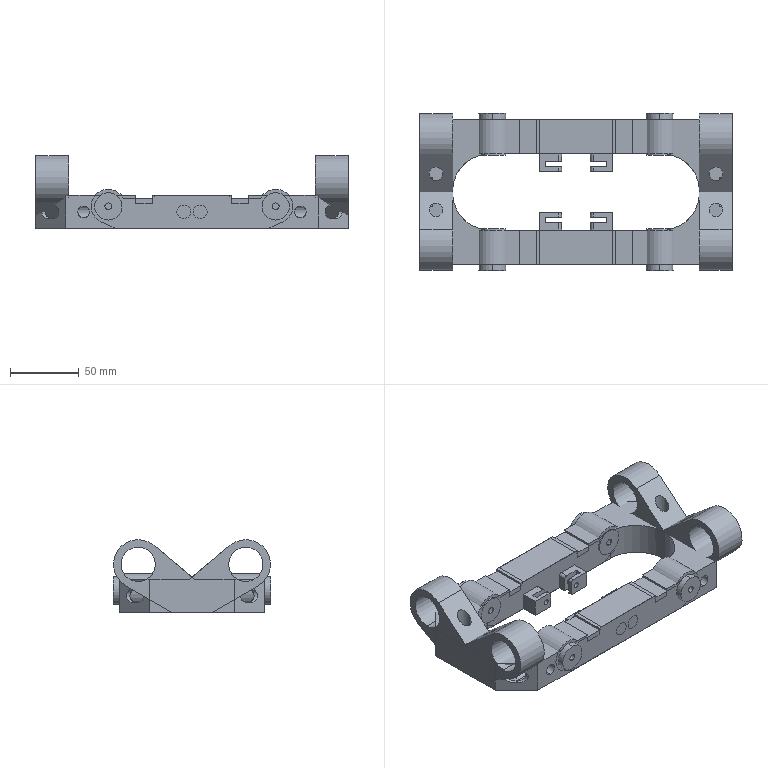CAM job | Mastercam | 3-axis milling, 5-axis milling, drilling, other | part box 228 x 114.503 x 53 mm | stock box 238 x 120 x 53 mm
Tools:
tool_number,name,type,diameter_mm,corner_radius_mm,flutes,flute_length_mm,overall_length_mm,shoulder_length_mm,holder_diameter_mm,length_offset,diameter_offset,default_rpm,default_feed_mm_min,default_plunge_mm_min,coolant
1,50 Slot Mill or Saw,slot mill,50,0,4,4,50,6,50,1,1,1000,150,600,COOL_OFF
1,2.5 Drill,drill,2.5,0,2,25,50,40,50,1,1,1200,70,600,COOL_OFF
2,4.2 Drill,drill,4.2,0,2,25,50,40,50,2,2,1000,100,600,COOL_OFF
2,4.1 Drill,drill,4.1,0,2,25,50,40,50,2,2,1500,100,600,COOL_OFF
3,10 Ball Mill / Bull Nose Mill,ball end mill,10,5,4,25,200,30,50,3,3,5000,1000,600,COOL_OFF
3,50 Flat End Mill,end mill,50,0,4,25,75,25,50,3,3,1400,200,600,COOL_OFF
4,4 Ball Mill / Bull Nose Mill,ball end mill,4,2,4,25,100,30,50,4,4,5000,1500,600,COOL_OFF
5,5 Drill,drill,5,0,2,25,50,40,50,5,5,1300,100,600,COOL_OFF
5,5 Drill,drill,5,0,2,25,50,40,50,5,5,1300,100,600,COOL_OFF
6,6 Flat End Mill,end mill,6,0,4,25,75,25,50,6,6,8000,3000,600,COOL_OFF
6,6 Flat End Mill,end mill,6,0,4,25,75,25,50,6,6,8000,3000,600,COOL_OFF
7,6 Chamfer Mill,chamfer mill,6,0,4,25,75,30,50,7,7,5000,1500,600,COOL_OFF
7,6 Chamfer Mill,chamfer mill,6,0,4,25,75,30,50,7,7,5000,1500,600,COOL_OFF
9,10 Drill,drill,10,0,2,25,200,40,50,9,9,1100,100,600,COOL_OFF
9,10 Drill,drill,10,0,2,25,200,40,50,9,9,1100,100,600,COOL_OFF
10,10 Flat End Mill,end mill,10,0,4,25,75,25,50,10,10,8500,6000,600,COOL_OFF
10,10 Flat End Mill,end mill,10,0,4,25,75,25,50,10,10,8500,6000,600,COOL_OFF
11,10 Drill,drill,10,0,2,25,200,40,50,11,11,600,80,600,COOL_OFF
11,10 Drill,drill,10,0,2,25,200,40,50,11,11,600,80,600,COOL_OFF
12,12 Flat End Mill,end mill,12,0,4,25,75,25,50,12,12,8000,6000,600,COOL_OFF
12,12 Flat End Mill,end mill,12,0,4,25,75,25,50,12,12,8000,6000,600,COOL_OFF
13,10 Bull Nose Mill,bull end mill,10,1,4,25,100,25,50,13,13,8000,4000,600,COOL_OFF
16,16 Flat End Mill,end mill,16,0,4,25,75,25,50,16,16,8250,4000,600,COOL_OFF
16,16 Flat End Mill,end mill,16,0,4,25,75,25,50,16,16,8250,4000,600,COOL_OFF
17,5 Ball Mill / Bull Nose Mill,ball end mill,5,2.5,4,25,100,30,50,17,17,5000,1500,600,COOL_OFF
17,5 Ball Mill / Bull Nose Mill,ball end mill,5,2.5,4,25,100,30,50,17,17,5000,1500,600,COOL_OFF
23,50 Flat End Mill,end mill,50,0,4,25,75,25,50,23,23,5000,4000,600,COOL_OFF
23,50 Flat End Mill,end mill,50,0,4,25,75,25,50,23,23,5000,4000,600,COOL_OFF
24,100 Flat End Mill,end mill,100,0,4,25,75,25,50,24,24,4000,1200,600,COOL_OFF
24,100 Flat End Mill,end mill,100,0,4,25,75,25,50,24,24,4000,1200,600,COOL_OFF
Operations:
seq,operation,operation_type,tool_number,tool_name,tool_diameter_mm,spindle_rpm,feed_mm_min,plunge_mm_min,retract_mm_min,cycle_time_s,wcs,posted,nc_file
1,Facing - [WCS: Plane] - [Tplane: Plane],Facing,24,100 Flat End Mill,100,4000,1200,600,1200,38.489,Plane,yes,1.nc
2,2D High Speed (2D Dynamic Mill) - [WCS: Plane] - [Tplane: Plane],HighSpeed2D,16,16 Flat End Mill,16,8250,4000,600,1200,119.906,Plane,yes,1.nc
3,Contour (2D) - [WCS: Plane] - [Tplane: Plane],Contour,16,16 Flat End Mill,16,5000,1000,600,1200,92.313,Plane,yes,1.nc
4,Contour (2D chamfer) - [WCS: Plane] - [Tplane: Plane],Contour,7,6 Chamfer Mill,6,5000,1500,600,1200,28.973,Plane,yes,1.nc
5,Facing - [WCS: Plane-4] - [Tplane: Plane-4],Facing,24,100 Flat End Mill,100,5000,3000,600,1200,65.426,Plane-4,yes,1.nc
6,Facing - [WCS: Plane-4] - [Tplane: Plane-4],Facing,24,100 Flat End Mill,100,5000,1000,600,1200,46.149,Plane-4,yes,1.nc
7,Drill/Counterbore - [WCS: Plane-4] - [Tplane: Plane-4],Drill,7,6 Chamfer Mill,6,5000,300,600,1200,1.67,Plane-4,yes,1.nc
8,Peck Drill - [WCS: Plane-4] - [Tplane: Plane-4],Drill,11,10 Drill,10,1200,150,600,1200,47.946,Plane-4,yes,1.nc
9,Contour (2D chamfer) - [WCS: Plane-4] - [Tplane: Plane-4],Contour,7,6 Chamfer Mill,6,5000,1500,600,1200,33.878,Plane-4,yes,1.nc
10,Contour (2D) - [WCS: Plane-2] - [Tplane: Plane-2],Contour,23,50 Flat End Mill,50,5000,4000,600,1200,376.188,Plane-2,yes,1.nc
11,Contour (Remachining) - [WCS: Plane-2] - [Tplane: Plane-2],Contour,10,10 Flat End Mill,10,8000,4000,600,1200,22.001,Plane-2,yes,1.nc
12,Contour (2D) - [WCS: Plane-2] - [Tplane: Plane-2],Contour,10,10 Flat End Mill,10,6000,1000,600,1200,46.662,Plane-2,yes,1.nc
13,Contour (Ramp) - [WCS: Plane-2] - [Tplane: Plane-2],Contour,10,10 Flat End Mill,10,8000,4000,600,1200,56.103,Plane-2,yes,1.nc
14,Contour (Ramp) - [WCS: Plane-2] - [Tplane: Plane-2],Contour,10,10 Flat End Mill,10,8000,1000,600,1200,19.219,Plane-2,yes,1.nc
15,Drill/Counterbore - [WCS: Plane-2] - [Tplane: Plane-2],Drill,7,6 Chamfer Mill,6,5000,300,600,1200,0.835,Plane-2,yes,1.nc
16,Peck Drill - [WCS: Plane-2] - [Tplane: Plane-2],Drill,11,10 Drill,10,1000,100,600,1200,28.243,Plane-2,yes,1.nc
17,Manual Entry (G0G90G54X-300.),ManualEntry,,,,0,0,0,0,0,Plane,yes,1.nc
18,Peck Drill - [WCS: Plane-2] - [Tplane: Plane-2],Drill,9,10 Drill,10,600,80,600,1200,116.677,Plane-2,yes,1.nc
19,Manual Entry (G0G90G54X-300.),ManualEntry,,,,0,0,0,0,0,Plane,yes,1.nc
20,Contour (2D chamfer) - [WCS: Plane-2] - [Tplane: Plane-2],Contour,7,6 Chamfer Mill,6,5000,1500,600,1200,19.89,Plane-2,yes,1.nc
21,Transform/Rotate Rotate About Point/Toolplane/Geometry,XForm,,,,0,0,0,0,685.819,Plane-2,yes,1.nc
22,Stock model - [WCS: Top] - [Tplane: Plane] - 1,139,,,,0,0,0,0,0,Top,yes,1.nc|2.nc|3.nc
23,2D High Speed (2D Area Mill) - [WCS: Plane-3] - [Tplane: Plane-3],HighSpeed2D,12,12 Flat End Mill,12,8500,6000,600,1200,76.463,Plane-3,yes,1.nc
24,Contour (Ramp) - [WCS: Plane-3] - [Tplane: Plane-3],Contour,12,12 Flat End Mill,12,8000,6000,600,1200,6.551,Plane-3,yes,1.nc
25,Contour (2D) - [WCS: Plane-3] - [Tplane: Plane-3],Contour,12,12 Flat End Mill,12,8000,1000,600,1200,8.109,Plane-3,yes,1.nc
26,2D High Speed (2D Area Mill) - [WCS: Plane-3] - [Tplane: Plane-3],HighSpeed2D,12,12 Flat End Mill,12,8500,1500,600,1200,47.681,Plane-3,yes,1.nc
27,Drill/Counterbore - [WCS: Plane-3] - [Tplane: Plane-3],Drill,7,6 Chamfer Mill,6,5000,300,600,1200,3.381,Plane-3,yes,1.nc
28,Peck Drill - [WCS: Plane-3] - [Tplane: Plane-3],Drill,5,5 Drill,5,1300,100,600,1200,26.184,Plane-3,yes,1.nc
29,Peck Drill - [WCS: Plane-3] - [Tplane: Plane-3],Drill,11,10 Drill,10,600,80,600,1200,67.7,Plane-3,yes,1.nc
30,Peck Drill - [WCS: Plane-3] - [Tplane: Plane-3],Drill,11,10 Drill,10,1100,100,600,1200,14.333,Plane-3,yes,1.nc
31,Contour (Ramp) - [WCS: Plane-3] - [Tplane: Plane-3],Contour,6,6 Flat End Mill,6,8000,3000,600,1200,5.394,Plane-3,yes,1.nc
32,Contour (2D chamfer) - [WCS: Plane-3] - [Tplane: Plane-3],Contour,7,6 Chamfer Mill,6,5000,1500,600,1200,14.165,Plane-3,yes,1.nc
33,Contour (2D chamfer) - [WCS: Plane-3] - [Tplane: Plane-3],Contour,7,6 Chamfer Mill,6,5000,1500,600,1200,20.962,Plane-3,yes,1.nc
34,Transform/Rotate Rotate About Point/Toolplane/NCI,XForm,,,,0,0,0,0,290.923,Plane,yes,1.nc
35,Stock model - [WCS: Top] - [Tplane: Plane-3] - 2,139,,,,0,0,0,0,0,Top,yes,1.nc|2.nc|3.nc
36,Contour (Ramp) - [WCS: Plane-1] - [Tplane: Plane-1],Contour,23,50 Flat End Mill,50,5000,4000,600,1200,172.897,Plane-1,yes,1.nc
37,Contour (2D) - [WCS: Plane-1] - [Tplane: Plane-1],Contour,10,10 Flat End Mill,10,6000,1000,600,1200,25.422,Plane-1,yes,1.nc
38,Contour (Ramp) - [WCS: Plane-1] - [Tplane: Plane-1],Contour,6,6 Flat End Mill,6,8000,3000,600,1200,11.291,Plane-1,yes,1.nc
39,Contour (2D) - [WCS: Plane-1] - [Tplane: Plane-1],Contour,6,6 Flat End Mill,6,8000,1000,600,1200,12.906,Plane-1,yes,1.nc
40,Contour (2D chamfer) - [WCS: Plane-1] - [Tplane: Plane-1],Contour,7,6 Chamfer Mill,6,5000,1500,600,1200,13.542,Plane-1,yes,1.nc
41,Drill/Counterbore - [WCS: Plane-1] - [Tplane: Plane-1],Drill,7,6 Chamfer Mill,6,5000,300,600,1200,3.095,Plane-1,yes,1.nc
42,Stock model - [WCS: Top] - [Tplane: Plane-1] - 3,139,,,,0,0,0,0,0,Top,yes,1.nc|2.nc|3.nc
43,Contour (Ramp) - [WCS: Plane] - [Tplane: Plane],Contour,24,100 Flat End Mill,100,5000,4000,600,1200,242.961,Plane,yes,1.nc
44,2D High Speed (2D Area Mill) - [WCS: Plane] - [Tplane: Plane],HighSpeed2D,12,12 Flat End Mill,12,8500,5000,600,1200,251.096,Plane,yes,1.nc
45,2D High Speed (2D Area Mill) - [WCS: Plane] - [Tplane: Plane],HighSpeed2D,12,12 Flat End Mill,12,8500,1200,600,1200,126.788,Plane,yes,1.nc
46,Contour (Ramp) - [WCS: Plane] - [Tplane: Plane],Contour,10,10 Flat End Mill,10,8500,6000,600,1200,15.497,Plane,yes,1.nc
47,Contour (2D) - [WCS: Plane] - [Tplane: Plane],Contour,10,10 Flat End Mill,10,8500,1000,600,1200,11.429,Plane,yes,1.nc
48,Contour (Ramp) - [WCS: Plane] - [Tplane: Plane],Contour,12,12 Flat End Mill,12,8000,6000,600,1200,6.911,Plane,yes,1.nc
49,Contour (2D) - [WCS: Plane] - [Tplane: Plane],Contour,12,12 Flat End Mill,12,8000,1000,600,1200,11.582,Plane,yes,1.nc
50,Contour (2D chamfer) - [WCS: Plane] - [Tplane: Plane],Contour,7,6 Chamfer Mill,6,5000,1500,600,1200,8.268,Plane,yes,1.nc
51,Contour (2D chamfer) - [WCS: Plane] - [Tplane: Plane],Contour,7,6 Chamfer Mill,6,5000,1500,600,1200,12.882,Plane,yes,1.nc
52,Ruled - [WCS: Plane] - [Tplane: Plane],Ruled,12,12 Flat End Mill,12,8000,4000,2000,1200,23.404,Plane,yes,1.nc
53,Ruled - [WCS: Plane] - [Tplane: Plane],Ruled,12,12 Flat End Mill,12,8000,4000,2000,1200,23.404,Plane,yes,1.nc
54,Surface Finish Flowline - [WCS: Plane] - [Tplane: Plane],MultiSurfaceFinishFlowline,13,10 Bull Nose Mill,10,8000,4000,600,1200,77.618,Plane,yes,1.nc
55,Surface Finish Flowline - [WCS: Plane] - [Tplane: Plane],MultiSurfaceFinishFlowline,13,10 Bull Nose Mill,10,8000,4000,600,1200,77.618,Plane,yes,1.nc
56,Deburr 5-axis - [WCS: Plane] - [Tplane: Plane],459,17,5 Ball Mill / Bull Nose Mill,5,5000,1500,600,1200,29.492,Plane,yes,1.nc
57,Drill/Counterbore - [WCS: Plane] - [Tplane: Plane],Drill,7,6 Chamfer Mill,6,5000,300,600,1200,5.169,Plane,yes,1.nc
58,Stock model - [WCS: Top] - [Tplane: Plane] - 4,139,,,,0,0,0,0,0,Top,yes,1.nc|2.nc|3.nc
59,Contour (2D) - [WCS: Plane-5] - [Tplane: Plane-5],Contour,16,16 Flat End Mill,16,5000,1000,600,1200,49.081,Plane-5,yes,1.nc
60,Contour (2D) - [WCS: Plane-5] - [Tplane: Plane-4],Contour,16,16 Flat End Mill,16,6000,4000,600,1200,326.038,Plane-5,yes,1.nc
61,Contour (2D) - [WCS: Plane-5] - [Tplane: Plane-4],Contour,16,16 Flat End Mill,16,6000,1000,600,1200,63.018,Plane-5,yes,1.nc
62,Contour (Ramp) - [WCS: Plane-5] - [Tplane: Plane-4],Contour,16,16 Flat End Mill,16,6000,4000,600,1200,259.668,Plane-5,yes,1.nc
63,Deburr 5-axis - [WCS: Plane-5] - [Tplane: Plane-5],459,17,5 Ball Mill / Bull Nose Mill,5,5000,1500,600,1200,22.138,Plane-5,yes,1.nc
64,Stock model - [WCS: Top] - [Tplane: Plane-4] - 5,139,,,,0,0,0,0,0,Top,yes,1.nc|2.nc|3.nc
65,Facing - [WCS: Plane-4] - [Tplane: Plane-4],Facing,24,100 Flat End Mill,100,5000,3000,600,1200,65.426,Plane-4,yes,1.nc
66,Facing - [WCS: Plane-4] - [Tplane: Plane-4],Facing,24,100 Flat End Mill,100,5000,1000,600,1200,46.149,Plane-4,yes,1.nc
67,Drill/Counterbore - [WCS: Plane-4] - [Tplane: Plane-4],Drill,7,6 Chamfer Mill,6,5000,300,600,1200,1.67,Plane-4,yes,1.nc
68,Peck Drill - [WCS: Plane-4] - [Tplane: Plane-4],Drill,11,10 Drill,10,1200,150,600,1200,47.946,Plane-4,yes,1.nc
69,Contour (2D chamfer) - [WCS: Plane-4] - [Tplane: Plane-4],Contour,7,6 Chamfer Mill,6,5000,1500,600,1200,33.878,Plane-4,yes,1.nc
70,Contour (Ramp) - [WCS: Plane-2] - [Tplane: Plane-2],Contour,23,50 Flat End Mill,50,5000,4000,600,1200,356.8,Plane-2,yes,1.nc
71,Contour (Remachining) - [WCS: Plane-2] - [Tplane: Plane-2],Contour,10,10 Flat End Mill,10,8000,4000,600,1200,21.855,Plane-2,yes,1.nc
72,Contour (2D) - [WCS: Plane-2] - [Tplane: Plane-2],Contour,10,10 Flat End Mill,10,6000,1000,600,1200,46.67,Plane-2,yes,1.nc
73,Contour (Ramp) - [WCS: Plane-2] - [Tplane: Plane-2],Contour,10,10 Flat End Mill,10,8000,4000,600,1200,56.103,Plane-2,yes,1.nc
74,Contour (Ramp) - [WCS: Plane-2] - [Tplane: Plane-2],Contour,10,10 Flat End Mill,10,8000,1000,600,1200,19.219,Plane-2,yes,1.nc
75,Drill/Counterbore - [WCS: Plane-2] - [Tplane: Plane-2],Drill,7,6 Chamfer Mill,6,5000,300,600,1200,0.835,Plane-2,yes,1.nc
76,Peck Drill - [WCS: Plane-2] - [Tplane: Plane-2],Drill,11,10 Drill,10,1000,100,600,1200,28.243,Plane-2,yes,1.nc
77,Manual Entry (G0G90G54X-300.),ManualEntry,,,,0,0,0,0,0,Plane,yes,1.nc
78,Peck Drill - [WCS: Plane-2] - [Tplane: Plane-2],Drill,9,10 Drill,10,600,80,600,1200,116.677,Plane-2,yes,1.nc
79,Manual Entry (G0G90G54X-300.),ManualEntry,,,,0,0,0,0,0,Plane,yes,1.nc
80,Contour (2D chamfer) - [WCS: Plane-2] - [Tplane: Plane-2],Contour,7,6 Chamfer Mill,6,5000,1500,600,1200,19.89,Plane-2,yes,1.nc
81,2D High Speed (2D Area Mill) - [WCS: Plane-3] - [Tplane: Plane-3],HighSpeed2D,12,12 Flat End Mill,12,8500,6000,600,1200,76.465,Plane-3,yes,1.nc
82,Contour (Ramp) - [WCS: Plane-3] - [Tplane: Plane-3],Contour,12,12 Flat End Mill,12,8000,6000,600,1200,6.551,Plane-3,yes,1.nc
83,Contour (2D) - [WCS: Plane-3] - [Tplane: Plane-3],Contour,12,12 Flat End Mill,12,8000,1000,600,1200,8.109,Plane-3,yes,1.nc
84,2D High Speed (2D Area Mill) - [WCS: Plane-3] - [Tplane: Plane-3],HighSpeed2D,12,12 Flat End Mill,12,8500,1500,600,1200,47.689,Plane-3,yes,1.nc
85,Drill/Counterbore - [WCS: Plane-3] - [Tplane: Plane-3],Drill,7,6 Chamfer Mill,6,5000,300,600,1200,3.117,Plane-3,yes,1.nc
86,Peck Drill - [WCS: Plane-3] - [Tplane: Plane-3],Drill,5,5 Drill,5,1300,100,600,1200,26.184,Plane-3,yes,1.nc
87,Peck Drill - [WCS: Plane-3] - [Tplane: Plane-3],Drill,11,10 Drill,10,600,80,600,1200,67.7,Plane-3,yes,1.nc
88,Peck Drill - [WCS: Plane-3] - [Tplane: Plane-3],Drill,11,10 Drill,10,1100,100,600,1200,14.333,Plane-3,yes,1.nc
89,Contour (Ramp) - [WCS: Plane-3] - [Tplane: Plane-3],Contour,6,6 Flat End Mill,6,8000,3000,600,1200,5.394,Plane-3,yes,1.nc
90,Contour (2D chamfer) - [WCS: Plane-3] - [Tplane: Plane-3],Contour,7,6 Chamfer Mill,6,5000,1500,600,1200,14.165,Plane-3,yes,1.nc
91,Contour (2D chamfer) - [WCS: Plane-3] - [Tplane: Plane-3],Contour,7,6 Chamfer Mill,6,5000,1500,600,1200,20.928,Plane-3,yes,1.nc
92,Contour (Ramp) - [WCS: Plane-1] - [Tplane: Plane-1],Contour,23,50 Flat End Mill,50,5000,4000,600,1200,172.897,Plane-1,yes,1.nc
93,Contour (2D) - [WCS: Plane-1] - [Tplane: Plane-1],Contour,10,10 Flat End Mill,10,6000,1000,600,1200,25.422,Plane-1,yes,1.nc
94,Contour (Ramp) - [WCS: Plane-1] - [Tplane: Plane-1],Contour,6,6 Flat End Mill,6,8000,3000,600,1200,11.291,Plane-1,yes,1.nc
95,Contour (2D) - [WCS: Plane-1] - [Tplane: Plane-1],Contour,6,6 Flat End Mill,6,8000,1000,600,1200,12.906,Plane-1,yes,1.nc
96,Contour (2D chamfer) - [WCS: Plane-1] - [Tplane: Plane-1],Contour,7,6 Chamfer Mill,6,5000,1500,600,1200,13.542,Plane-1,yes,1.nc
97,Drill/Counterbore - [WCS: Plane-1] - [Tplane: Plane-1],Drill,7,6 Chamfer Mill,6,5000,300,600,1200,3.095,Plane-1,yes,1.nc
98,Contour (Ramp) - [WCS: Plane] - [Tplane: Plane],Contour,24,100 Flat End Mill,100,5000,4000,600,1200,242.961,Plane,yes,1.nc
99,2D High Speed (2D Area Mill) - [WCS: Plane] - [Tplane: Plane],HighSpeed2D,12,12 Flat End Mill,12,8500,5000,600,1200,250.798,Plane,yes,1.nc
100,2D High Speed (2D Area Mill) - [WCS: Plane] - [Tplane: Plane],HighSpeed2D,12,12 Flat End Mill,12,8500,1200,600,1200,126.822,Plane,yes,1.nc
101,Contour (Ramp) - [WCS: Plane] - [Tplane: Plane],Contour,10,10 Flat End Mill,10,8500,6000,600,1200,15.497,Plane,yes,1.nc
102,Contour (2D) - [WCS: Plane] - [Tplane: Plane],Contour,10,10 Flat End Mill,10,8500,1000,600,1200,11.429,Plane,yes,1.nc
103,Contour (Ramp) - [WCS: Plane] - [Tplane: Plane],Contour,12,12 Flat End Mill,12,8000,6000,600,1200,6.911,Plane,yes,1.nc
104,Contour (2D) - [WCS: Plane] - [Tplane: Plane],Contour,12,12 Flat End Mill,12,8000,1000,600,1200,11.582,Plane,yes,1.nc
105,Contour (2D chamfer) - [WCS: Plane] - [Tplane: Plane],Contour,7,6 Chamfer Mill,6,5000,1500,600,1200,8.268,Plane,yes,1.nc
106,Contour (2D chamfer) - [WCS: Plane] - [Tplane: Plane],Contour,7,6 Chamfer Mill,6,5000,1500,600,1200,12.882,Plane,yes,1.nc
107,Ruled - [WCS: Plane] - [Tplane: Plane],Ruled,12,12 Flat End Mill,12,8000,4000,4000,1200,22.287,Plane,yes,1.nc
108,Ruled - [WCS: Plane] - [Tplane: Plane],Ruled,12,12 Flat End Mill,12,8000,4000,4000,1200,22.287,Plane,yes,1.nc
109,Surface Finish Flowline - [WCS: Plane] - [Tplane: Plane],MultiSurfaceFinishFlowline,13,10 Bull Nose Mill,10,8000,2000,600,1200,310.124,Plane,yes,1.nc
110,Deburr 5-axis - [WCS: Plane] - [Tplane: Plane],459,17,5 Ball Mill / Bull Nose Mill,5,5000,1500,600,1200,30.372,Plane,yes,1.nc
111,Drill/Counterbore - [WCS: Plane] - [Tplane: Plane],Drill,7,6 Chamfer Mill,6,5000,300,600,1200,5.169,Plane,yes,1.nc
112,Contour (2D) - [WCS: Plane-5] - [Tplane: Plane-5],Contour,16,16 Flat End Mill,16,5000,1000,600,1200,49.081,Plane-5,yes,1.nc
113,Contour (2D) - [WCS: Plane-5] - [Tplane: Plane-4],Contour,16,16 Flat End Mill,16,6000,4000,600,1200,326.081,Plane-5,yes,1.nc
114,Contour (2D) - [WCS: Plane-5] - [Tplane: Plane-4],Contour,16,16 Flat End Mill,16,6000,1000,600,1200,63.04,Plane-5,yes,1.nc
115,Contour (Ramp) - [WCS: Plane-5] - [Tplane: Plane-4],Contour,16,16 Flat End Mill,16,6000,4000,600,1200,188.091,Plane-5,yes,1.nc
116,Deburr 5-axis - [WCS: Plane-5] - [Tplane: Plane-4],459,17,5 Ball Mill / Bull Nose Mill,5,5000,1500,600,1200,25.436,Plane-5,yes,1.nc
117,2D High Speed (2D Area Mill) - [WCS: Plane-6] - [Tplane: Plane-6],HighSpeed2D,12,12 Flat End Mill,12,6000,6000,600,1200,212.363,Plane-6,yes,2.nc
118,2D High Speed (2D Area Mill) - [WCS: Plane-6] - [Tplane: Plane-6],HighSpeed2D,12,12 Flat End Mill,12,6000,1000,600,1200,31.766,Plane-6,yes,2.nc
119,Contour (2D) - [WCS: Plane-6] - [Tplane: Plane-6],Contour,12,12 Flat End Mill,12,6000,1000,600,1200,5.203,Plane-6,yes,2.nc
120,Contour (2D) - [WCS: Plane-6] - [Tplane: Plane-6],Contour,12,12 Flat End Mill,12,6000,1000,600,1200,8.051,Plane-6,yes,2.nc
121,Contour (2D) - [WCS: Plane-6] - [Tplane: Plane-6],Contour,12,12 Flat End Mill,12,6000,1000,600,1200,4.536,Plane-6,yes,2.nc
122,Contour (2D) - [WCS: Plane-6] - [Tplane: Plane-6],Contour,12,12 Flat End Mill,12,6000,1000,600,1200,5.32,Plane-6,yes,2.nc
123,Drill/Counterbore - [WCS: Plane-6] - [Tplane: Plane-6],Drill,7,6 Chamfer Mill,6,6000,300,600,1200,0.774,Plane-6,yes,2.nc
124,Contour (Ramp) - [WCS: Plane-6] - [Tplane: Plane-6],Contour,12,12 Flat End Mill,12,6000,6000,600,1200,47.827,Plane-6,yes,2.nc
125,Contour (2D) - [WCS: Plane-6] - [Tplane: Plane-6],Contour,12,12 Flat End Mill,12,6000,1000,600,1200,8.707,Plane-6,yes,2.nc
126,Deburr 5-axis - [WCS: Plane-6] - [Tplane: Plane-6],459,3,50 Flat End Mill,50,6000,1500,600,1200,27.102,Plane-6,yes,2.nc
127,Deburr 5-axis - [WCS: Plane-6] - [Tplane: Plane-6],459,4,4 Ball Mill / Bull Nose Mill,4,6000,1500,600,1200,6.266,Plane-6,yes,2.nc
128,2D High Speed (2D Area Mill) - [WCS: Plane-7] - [Tplane: Plane-7],HighSpeed2D,12,12 Flat End Mill,12,6000,6000,600,1200,212.304,Plane-7,yes,2.nc
129,2D High Speed (2D Area Mill) - [WCS: Plane-7] - [Tplane: Plane-7],HighSpeed2D,12,12 Flat End Mill,12,6000,1000,600,1200,32.214,Plane-7,yes,2.nc
130,Contour (2D) - [WCS: Plane-7] - [Tplane: Plane-7],Contour,12,12 Flat End Mill,12,6000,1000,600,1200,5.203,Plane-7,yes,2.nc
131,Contour (2D) - [WCS: Plane-7] - [Tplane: Plane-7],Contour,12,12 Flat End Mill,12,6000,1000,600,1200,8.051,Plane-7,yes,2.nc
132,Contour (2D) - [WCS: Plane-7] - [Tplane: Plane-7],Contour,12,12 Flat End Mill,12,6000,1000,600,1200,4.536,Plane-7,yes,2.nc
133,Contour (2D) - [WCS: Plane-7] - [Tplane: Plane-7],Contour,12,12 Flat End Mill,12,6000,1000,600,1200,5.32,Plane-7,yes,2.nc
134,Chamfer Drill - [WCS: Plane-7] - [Tplane: Plane-7],ChamferDrill,7,6 Chamfer Mill,6,6000,1500,600,1200,1.526,Plane-7,no,
135,Contour (2D) - [WCS: Plane-7] - [Tplane: Plane-7],Contour,1,2.5 Drill,2.5,6000,600,600,1200,12.625,Plane-7,no,
136,Contour (Ramp) - [WCS: Plane-7] - [Tplane: Plane-7],Contour,12,12 Flat End Mill,12,6000,6000,600,1200,47.827,Plane-7,yes,2.nc
137,Contour (2D) - [WCS: Plane-7] - [Tplane: Plane-7],Contour,12,12 Flat End Mill,12,6000,1000,600,1200,8.707,Plane-7,yes,2.nc
138,Deburr 5-axis - [WCS: Plane-7] - [Tplane: Plane-7],459,3,50 Flat End Mill,50,6000,1500,600,1200,24.941,Plane-7,yes,2.nc
139,Deburr 5-axis - [WCS: Plane-7] - [Tplane: Plane-7],459,4,4 Ball Mill / Bull Nose Mill,4,6000,1500,600,1200,10.622,Plane-7,yes,2.nc
140,Drill/Counterbore - [WCS: Plane-7] - [Tplane: Plane-7],Drill,7,6 Chamfer Mill,6,5000,200,600,1200,1.044,Plane-7,yes,2.nc
141,Peck Drill - [WCS: Plane-8] - [Tplane: Plane-8],Drill,1,2.5 Drill,2.5,1200,70,600,1200,18.239,Plane-8,yes,3.nc
142,Peck Drill - [WCS: Plane-8] - [Tplane: Plane-8],Drill,2,4.1 Drill,4.1,1000,100,600,1200,5.275,Plane-8,yes,3.nc
143,Contour (2D) - [WCS: Plane-8] - [Tplane: Plane-8],Contour,3,50 Flat End Mill,50,1400,200,600,1200,24.206,Plane-8,yes,3.nc
144,Peck Drill - [WCS: Plane-9] - [Tplane: Plane-9],Drill,1,2.5 Drill,2.5,1200,70,600,1200,18.239,Plane-9,yes,3.nc
145,Peck Drill - [WCS: Plane-9] - [Tplane: Plane-9],Drill,2,4.1 Drill,4.1,1000,100,600,1200,5.275,Plane-9,yes,3.nc
146,Contour (2D) - [WCS: Plane-9] - [Tplane: Plane-9],Contour,3,50 Flat End Mill,50,1400,50,600,1200,93.956,Plane-9,yes,3.nc